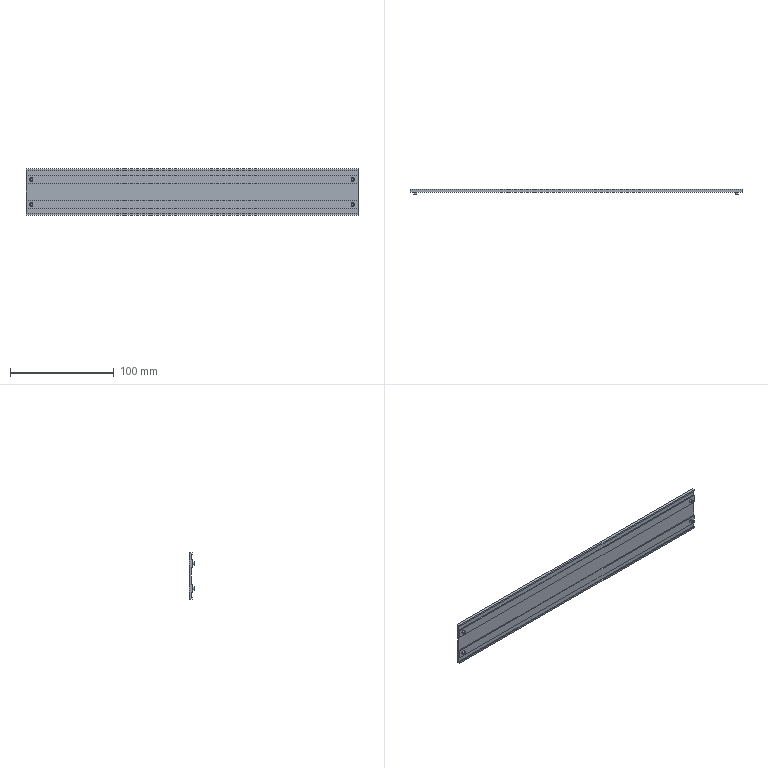Part | STEP file | C-KS50-300_c | 1 solid | 146 faces | box 320 x 5 x 45 mm | volume 26928 mm3 | plane 92 | cylinder 34 | cone 16 | torus 4 | commonest cylinder face diameters 0.8 x22 3 x4 3.5 x4 5.54 x4